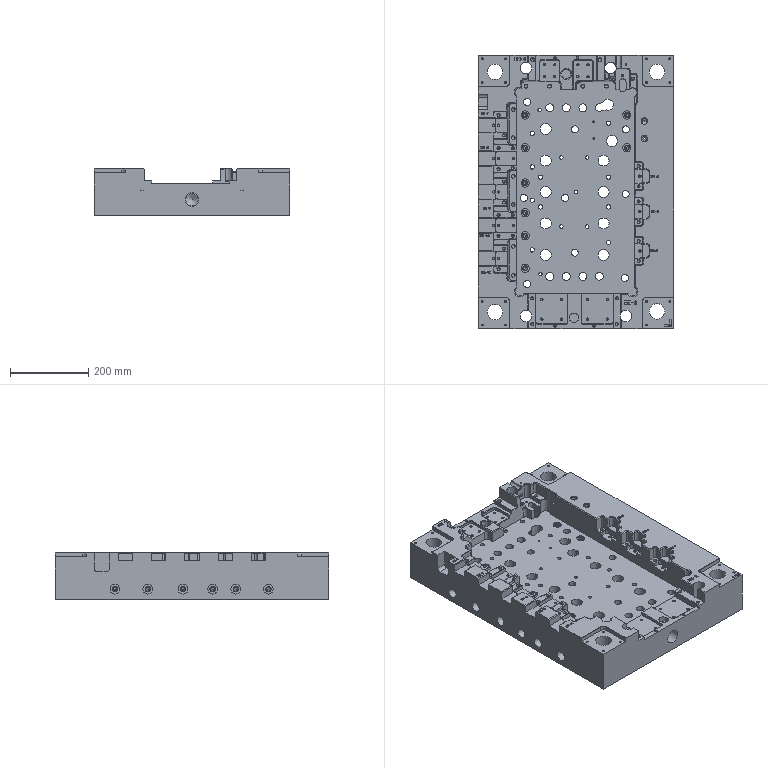Part | STEP file | solid 186 | 1 solid | 2049 faces | box 500 x 700 x 120 mm | volume 24510604 mm3 | plane 1144 | cylinder 536 | cone 237 | other 110 | spline 20 | torus 2 | commonest cylinder face diameters 10 x120 8 x70 6 x44 5 x43 6.7 x38 7 x26